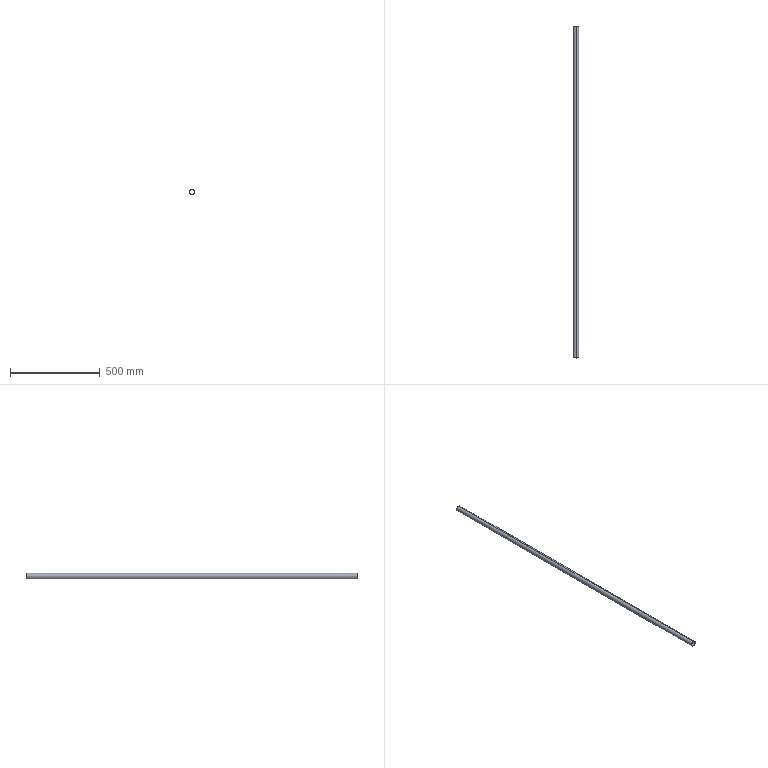Part | SolidWorks | features Sweep 1 | 1 solid | 6 faces | box 30 x 1846 x 30 mm | volume 324836 mm3 | cylinder 4 | plane 2 | commonest cylinder face diameters 26 x2 30 x2
STEP:
#1=CARTESIAN_POINT('',(0.,0.,-13.));
#2=VERTEX_POINT('',#1);
#3=CARTESIAN_POINT('',(0.,0.,13.));
#4=VERTEX_POINT('',#3);
#5=CARTESIAN_POINT('',(0.,0.,0.));
#6=DIRECTION('',(0.,1.,0.));
#7=DIRECTION('',(0.,0.,1.));
#8=AXIS2_PLACEMENT_3D('',#5,#6,#7);
#9=CIRCLE('',#8,13.);
#10=EDGE_CURVE('',#2,#4,#9,.T.);
#11=ORIENTED_EDGE('',*,*,#10,.F.);
#12=CARTESIAN_POINT('',(0.,1846.4,-13.));
#13=VERTEX_POINT('',#12);
#14=CARTESIAN_POINT('',(0.,0.,-13.));
#15=DIRECTION('',(0.,1.,0.));
#16=VECTOR('',#15,1000.);
#17=LINE('',#14,#16);
#18=EDGE_CURVE('',#2,#13,#17,.T.);
#19=ORIENTED_EDGE('',*,*,#18,.T.);
#20=CARTESIAN_POINT('',(0.,1846.4,13.));
#21=VERTEX_POINT('',#20);
#22=CARTESIAN_POINT('',(0.,1846.4,0.));
#23=DIRECTION('',(0.,1.,0.));
#24=DIRECTION('',(0.,0.,1.));
#25=AXIS2_PLACEMENT_3D('',#22,#23,#24);
#26=CIRCLE('',#25,13.);
#27=EDGE_CURVE('',#13,#21,#26,.T.);
#28=ORIENTED_EDGE('',*,*,#27,.T.);
#29=CARTESIAN_POINT('',(0.,0.,13.));
#30=DIRECTION('',(0.,1.,0.));
#31=VECTOR('',#30,1000.);
#32=LINE('',#29,#31);
#33=EDGE_CURVE('',#4,#21,#32,.T.);
#34=ORIENTED_EDGE('',*,*,#33,.F.);
#35=EDGE_LOOP('',(#11,#19,#28,#34));
#36=FACE_OUTER_BOUND('',#35,.T.);
#37=CARTESIAN_POINT('',(0.,0.,0.));
#38=DIRECTION('',(0.,1.,0.));
#39=DIRECTION('',(0.,0.,1.));
#40=AXIS2_PLACEMENT_3D('',#37,#38,#39);
#41=CYLINDRICAL_SURFACE('',#40,13.);
#42=ADVANCED_FACE('',(#36),#41,.F.);
#43=CARTESIAN_POINT('',(0.,0.,15.));
#44=VERTEX_POINT('',#43);
#45=CARTESIAN_POINT('',(0.,0.,-15.));
#46=VERTEX_POINT('',#45);
#47=CARTESIAN_POINT('',(0.,0.,0.));
#48=DIRECTION('',(0.,1.,0.));
#49=DIRECTION('',(0.,0.,1.));
#50=AXIS2_PLACEMENT_3D('',#47,#48,#49);
#51=CIRCLE('',#50,15.);
#52=EDGE_CURVE('',#44,#46,#51,.T.);
#53=ORIENTED_EDGE('',*,*,#52,.T.);
#54=CARTESIAN_POINT('',(0.,1846.4,-15.));
#55=VERTEX_POINT('',#54);
#56=CARTESIAN_POINT('',(0.,0.,-15.));
#57=DIRECTION('',(0.,1.,0.));
#58=VECTOR('',#57,1000.);
#59=LINE('',#56,#58);
#60=EDGE_CURVE('',#46,#55,#59,.T.);
#61=ORIENTED_EDGE('',*,*,#60,.T.);
#62=CARTESIAN_POINT('',(0.,1846.4,15.));
#63=VERTEX_POINT('',#62);
#64=CARTESIAN_POINT('',(0.,1846.4,0.));
#65=DIRECTION('',(0.,1.,0.));
#66=DIRECTION('',(0.,0.,1.));
#67=AXIS2_PLACEMENT_3D('',#64,#65,#66);
#68=CIRCLE('',#67,15.);
#69=EDGE_CURVE('',#63,#55,#68,.T.);
#70=ORIENTED_EDGE('',*,*,#69,.F.);
#71=CARTESIAN_POINT('',(0.,0.,15.));
#72=DIRECTION('',(0.,1.,0.));
#73=VECTOR('',#72,1000.);
#74=LINE('',#71,#73);
#75=EDGE_CURVE('',#44,#63,#74,.T.);
#76=ORIENTED_EDGE('',*,*,#75,.F.);
#77=EDGE_LOOP('',(#53,#61,#70,#76));
#78=FACE_OUTER_BOUND('',#77,.T.);
#79=CARTESIAN_POINT('',(0.,0.,0.));
#80=DIRECTION('',(0.,1.,0.));
#81=DIRECTION('',(0.,0.,1.));
#82=AXIS2_PLACEMENT_3D('',#79,#80,#81);
#83=CYLINDRICAL_SURFACE('',#82,15.);
#84=ADVANCED_FACE('',(#78),#83,.T.);
#85=ORIENTED_EDGE('',*,*,#60,.F.);
#86=CARTESIAN_POINT('',(0.,0.,0.));
#87=DIRECTION('',(0.,1.,0.));
#88=DIRECTION('',(0.,0.,1.));
#89=AXIS2_PLACEMENT_3D('',#86,#87,#88);
#90=CIRCLE('',#89,15.);
#91=EDGE_CURVE('',#46,#44,#90,.T.);
#92=ORIENTED_EDGE('',*,*,#91,.T.);
#93=ORIENTED_EDGE('',*,*,#75,.T.);
#94=CARTESIAN_POINT('',(0.,1846.4,0.));
#95=DIRECTION('',(0.,1.,0.));
#96=DIRECTION('',(0.,0.,1.));
#97=AXIS2_PLACEMENT_3D('',#94,#95,#96);
#98=CIRCLE('',#97,15.);
#99=EDGE_CURVE('',#55,#63,#98,.T.);
#100=ORIENTED_EDGE('',*,*,#99,.F.);
#101=EDGE_LOOP('',(#85,#92,#93,#100));
#102=FACE_OUTER_BOUND('',#101,.T.);
#103=CARTESIAN_POINT('',(0.,0.,0.));
#104=DIRECTION('',(0.,1.,0.));
#105=DIRECTION('',(0.,0.,1.));
#106=AXIS2_PLACEMENT_3D('',#103,#104,#105);
#107=CYLINDRICAL_SURFACE('',#106,15.);
#108=ADVANCED_FACE('',(#102),#107,.T.);
#109=CARTESIAN_POINT('',(0.,1846.4,0.));
#110=DIRECTION('',(0.,1.,0.));
#111=DIRECTION('',(0.,0.,1.));
#112=AXIS2_PLACEMENT_3D('',#109,#110,#111);
#113=CIRCLE('',#112,13.);
#114=EDGE_CURVE('',#21,#13,#113,.T.);
#115=ORIENTED_EDGE('',*,*,#114,.F.);
#116=ORIENTED_EDGE('',*,*,#27,.F.);
#117=EDGE_LOOP('',(#115,#116));
#118=FACE_BOUND('',#117,.T.);
#119=ORIENTED_EDGE('',*,*,#69,.T.);
#120=ORIENTED_EDGE('',*,*,#99,.T.);
#121=EDGE_LOOP('',(#119,#120));
#122=FACE_OUTER_BOUND('',#121,.T.);
#123=CARTESIAN_POINT('',(0.,1846.4,0.));
#124=DIRECTION('',(0.,1.,0.));
#125=DIRECTION('',(0.,0.,1.));
#126=AXIS2_PLACEMENT_3D('',#123,#124,#125);
#127=PLANE('',#126);
#128=ADVANCED_FACE('',(#118,#122),#127,.T.);
#129=CARTESIAN_POINT('',(0.,0.,0.));
#130=DIRECTION('',(0.,1.,0.));
#131=DIRECTION('',(0.,0.,1.));
#132=AXIS2_PLACEMENT_3D('',#129,#130,#131);
#133=CIRCLE('',#132,13.);
#134=EDGE_CURVE('',#4,#2,#133,.T.);
#135=ORIENTED_EDGE('',*,*,#134,.T.);
#136=ORIENTED_EDGE('',*,*,#10,.T.);
#137=EDGE_LOOP('',(#135,#136));
#138=FACE_BOUND('',#137,.T.);
#139=ORIENTED_EDGE('',*,*,#52,.F.);
#140=ORIENTED_EDGE('',*,*,#91,.F.);
#141=EDGE_LOOP('',(#139,#140));
#142=FACE_OUTER_BOUND('',#141,.T.);
#143=CARTESIAN_POINT('',(0.,0.,0.));
#144=DIRECTION('',(0.,1.,0.));
#145=DIRECTION('',(0.,0.,1.));
#146=AXIS2_PLACEMENT_3D('',#143,#144,#145);
#147=PLANE('',#146);
#148=ADVANCED_FACE('',(#138,#142),#147,.F.);
#149=ORIENTED_EDGE('',*,*,#18,.F.);
#150=ORIENTED_EDGE('',*,*,#134,.F.);
#151=ORIENTED_EDGE('',*,*,#33,.T.);
#152=ORIENTED_EDGE('',*,*,#114,.T.);
#153=EDGE_LOOP('',(#149,#150,#151,#152));
#154=FACE_OUTER_BOUND('',#153,.T.);
#155=CARTESIAN_POINT('',(0.,0.,0.));
#156=DIRECTION('',(0.,1.,0.));
#157=DIRECTION('',(0.,0.,1.));
#158=AXIS2_PLACEMENT_3D('',#155,#156,#157);
#159=CYLINDRICAL_SURFACE('',#158,13.);
#160=ADVANCED_FACE('',(#154),#159,.F.);
#161=CLOSED_SHELL('',(#42,#84,#108,#128,#148,#160));
#162=MANIFOLD_SOLID_BREP('',#161);
#163=CARTESIAN_POINT('',(0.,0.,0.));
#164=DIRECTION('',(0.,0.,1.));
#165=DIRECTION('',(1.,0.,0.));
#166=AXIS2_PLACEMENT_3D('',#163,#164,#165);
#167=(LENGTH_UNIT()NAMED_UNIT(*)SI_UNIT(.MILLI.,.METRE.));
#168=UNCERTAINTY_MEASURE_WITH_UNIT(LENGTH_MEASURE(0.00001),#167,'','');
#169=(NAMED_UNIT(*)PLANE_ANGLE_UNIT()SI_UNIT($,.RADIAN.));
#170=(NAMED_UNIT(*)SI_UNIT($,.STERADIAN.)SOLID_ANGLE_UNIT());
#171=(GEOMETRIC_REPRESENTATION_CONTEXT(3)GLOBAL_UNCERTAINTY_ASSIGNED_CONTEXT((#168))GLOBAL_UNIT_ASSIGNED_CONTEXT((#167,#169,#170))REPRESENTATION_CONTEXT('',''));
#172=ADVANCED_BREP_SHAPE_REPRESENTATION('',(#162,#166),#171);